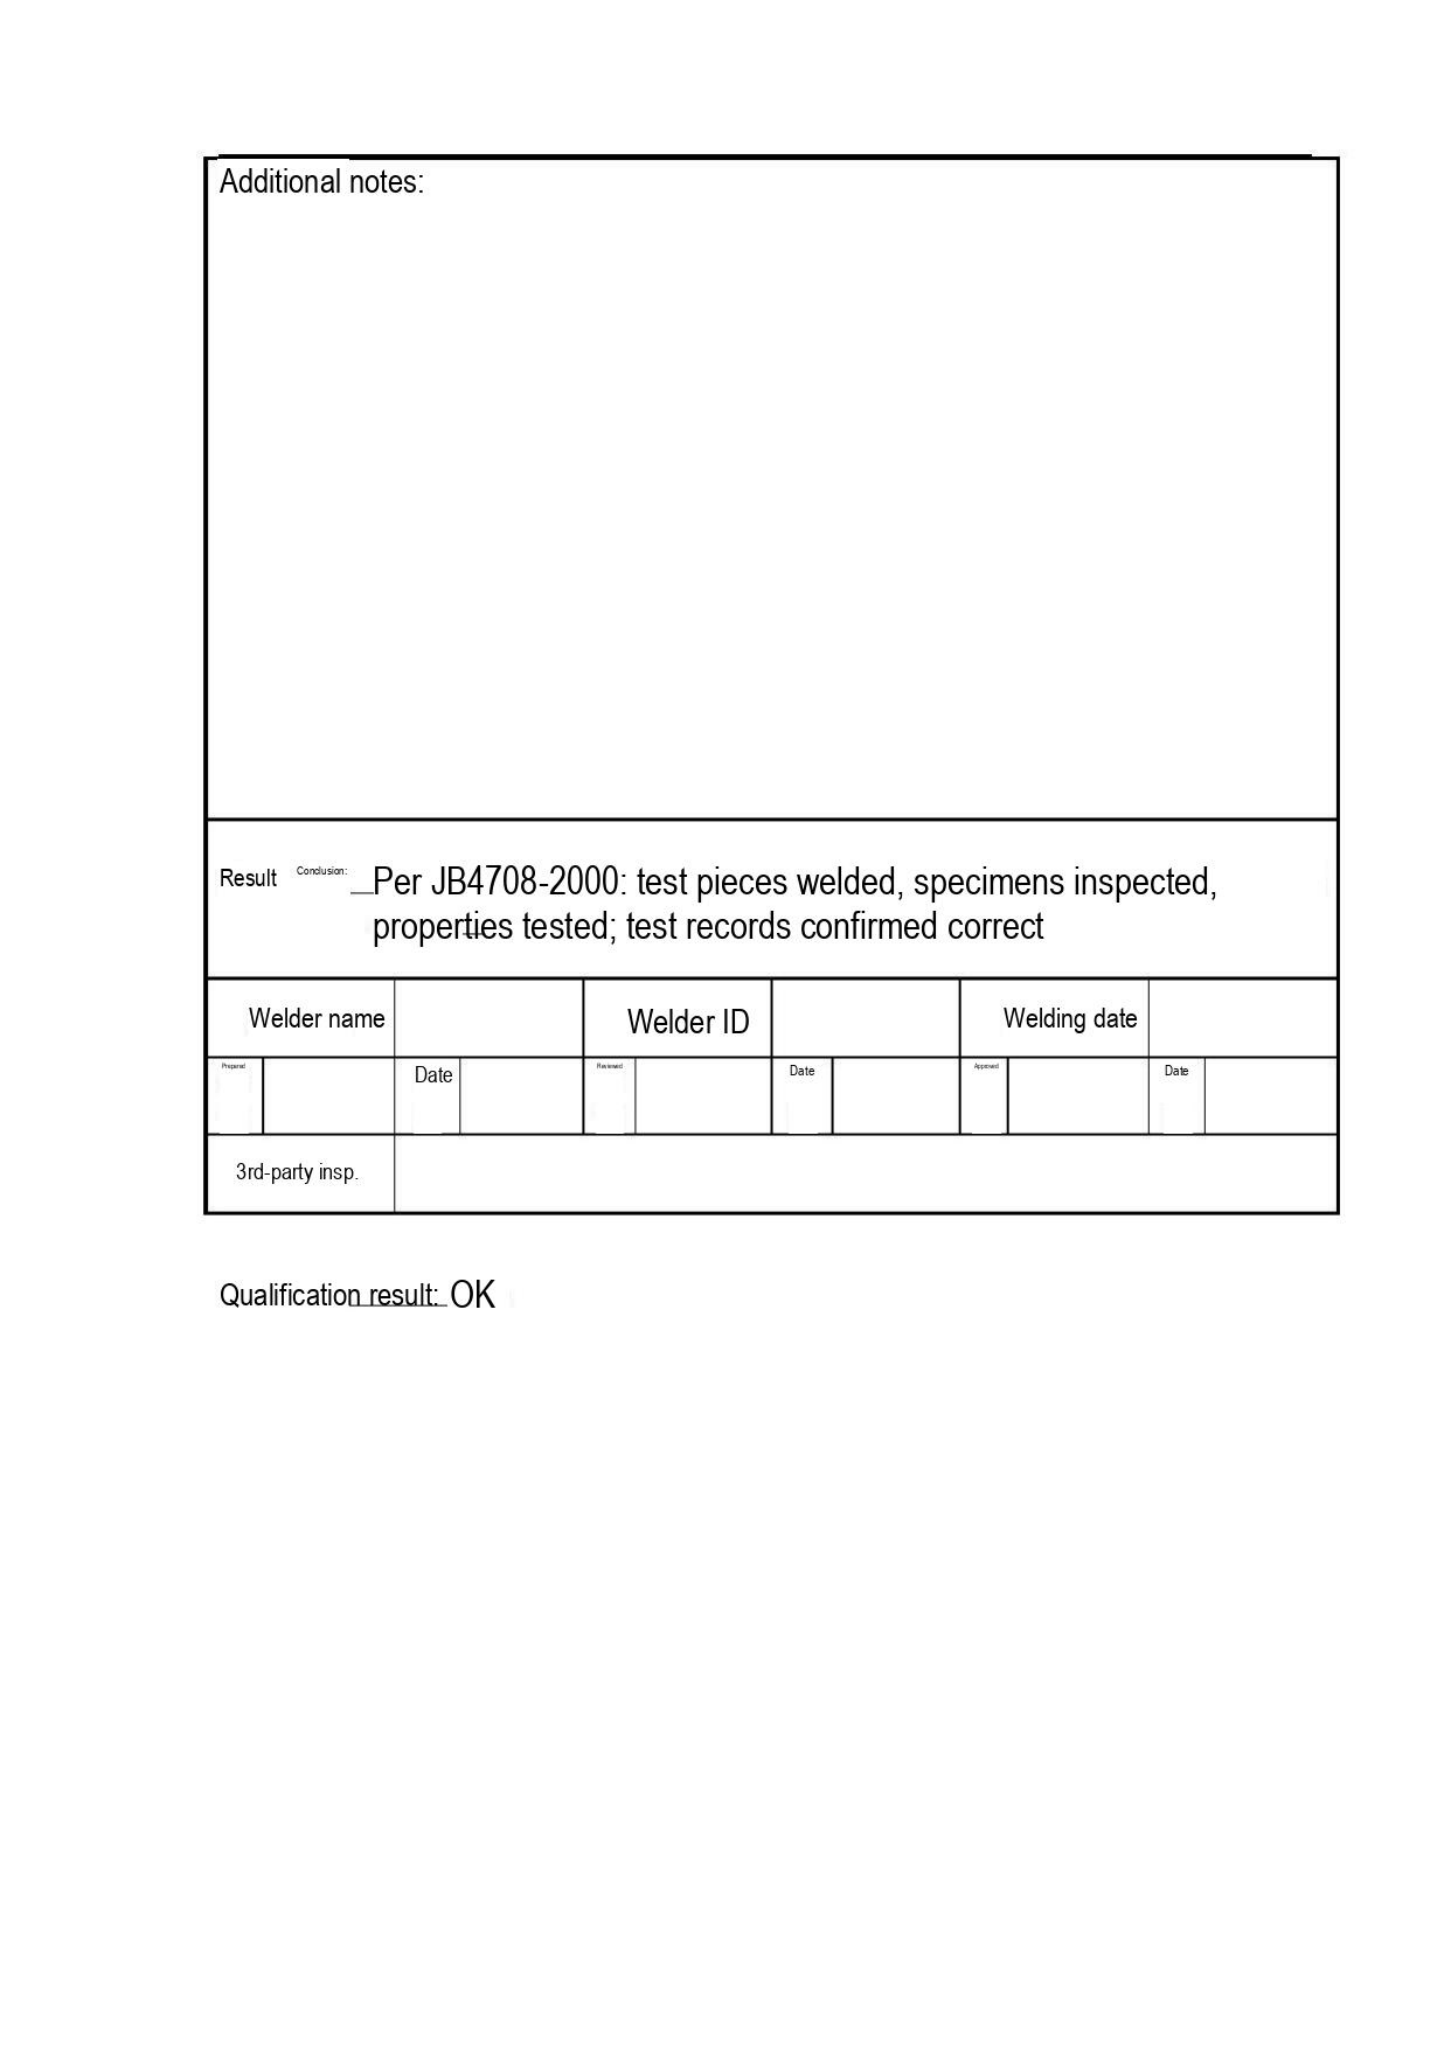Additional notes:

Result Conclusion: Per JB4708-2000: test pieces welded, specimens inspected, properties tested; test records confirmed correct

| Welder name | | Welder ID | | Welding date | |
|---|---|---|---|---|---|

| Prepared | | Date | | Reviewed | | Date | | Approved | | Date | |
|---|---|---|---|---|---|---|---|---|---|---|---|

| 3rd-party insp. | |
|---|---|

Qualification result: OK
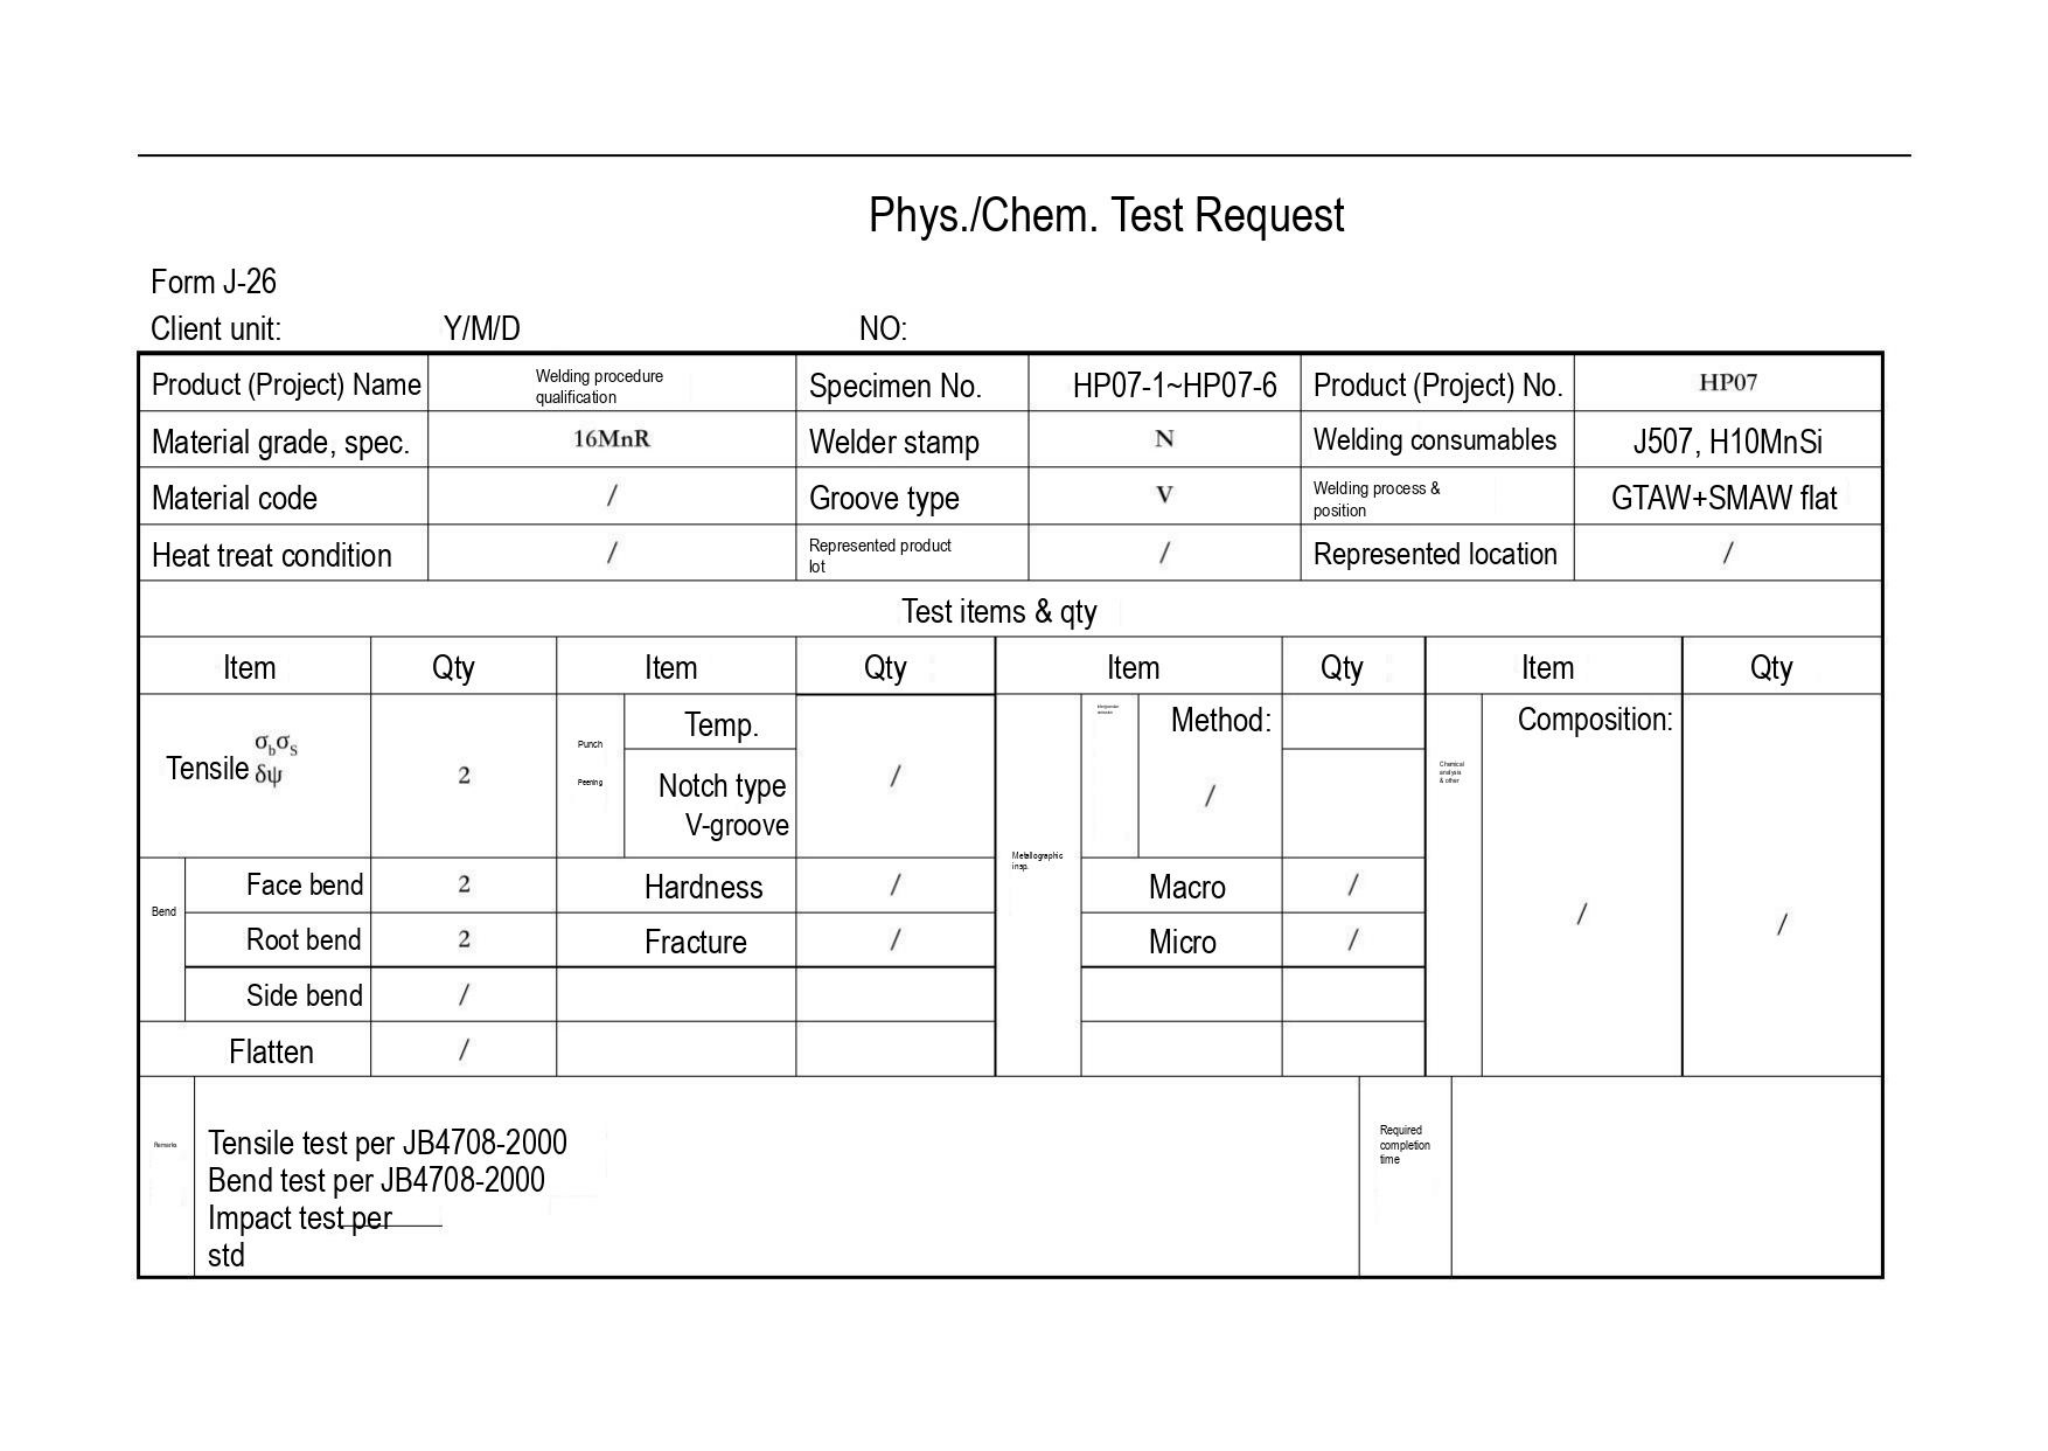# Phys./Chem. Test Request

Form J-26

Client unit: Y/M/D NO:

| Product (Project) Name | Welding procedure qualification | Specimen No. | HP07-1~HP07-6 | Product (Project) No. | HP07 |
|---|---|---|---|---|---|
| Material grade, spec. | 16MnR | Welder stamp | N | Welding consumables | J507, H10MnSi |
| Material code | / | Groove type | V | Welding process & position | GTAW+SMAW flat |
| Heat treat condition | / | Represented product lot | / | Represented location | / |

Test items & qty

| Item | Qty | Item | Qty | Item | Qty | Item | Qty |
|---|---|---|---|---|---|---|---|
| Tensile σbσs δψ | 2 | Punch Peening: Temp. / Notch type V-groove | / | Metallographic insp.: Method: / | | Chemical analysis & other: Composition: / | / |
| Bend: Face bend | 2 | Hardness | / | Macro | / | | |
| Bend: Root bend | 2 | Fracture | / | Micro | / | | |
| Bend: Side bend | / | | | | | | |
| Flatten | / | | | | | | |

| Remarks | Tensile test per JB4708-2000<br>Bend test per JB4708-2000<br>Impact test per \_\_\_\_\_ std | Required completion time | |
|---|---|---|---|